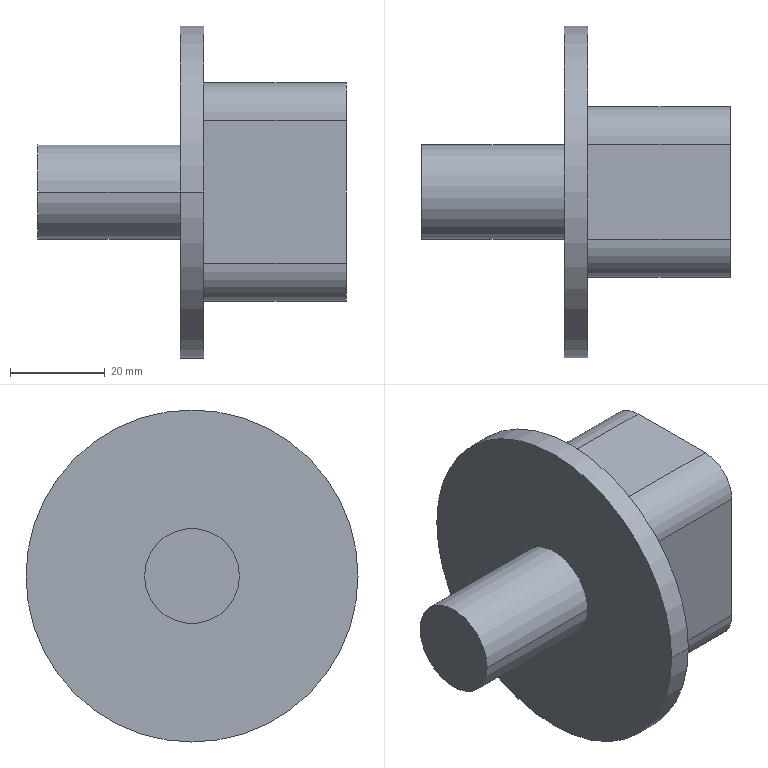Part | SolidWorks | features Extrusion 1, Revolution 1 | 1 solid | 16 faces | box 65 x 70 x 70 mm | volume 76699 mm3 | cylinder 8 | plane 8 | commonest cylinder face diameters 16 x4 20 x2 70 x2
STEP:
#1=CARTESIAN_POINT('',(-35.,-10.,0.));
#2=VERTEX_POINT('',#1);
#3=CARTESIAN_POINT('',(-35.,10.,0.));
#4=VERTEX_POINT('',#3);
#5=CARTESIAN_POINT('',(-35.,0.,0.));
#6=DIRECTION('',(-1.,0.,0.));
#7=DIRECTION('',(0.,-1.,0.));
#8=AXIS2_PLACEMENT_3D('',#5,#6,#7);
#9=CIRCLE('',#8,10.);
#10=EDGE_CURVE('',#2,#4,#9,.T.);
#11=ORIENTED_EDGE('',*,*,#10,.T.);
#12=CARTESIAN_POINT('',(-65.,10.,0.));
#13=VERTEX_POINT('',#12);
#14=CARTESIAN_POINT('',(-65.,10.,0.));
#15=DIRECTION('',(-1.,0.,0.));
#16=VECTOR('',#15,1000.);
#17=LINE('',#14,#16);
#18=EDGE_CURVE('',#4,#13,#17,.T.);
#19=ORIENTED_EDGE('',*,*,#18,.T.);
#20=CARTESIAN_POINT('',(-65.,-10.,0.));
#21=VERTEX_POINT('',#20);
#22=CARTESIAN_POINT('',(-65.,0.,0.));
#23=DIRECTION('',(-1.,0.,0.));
#24=DIRECTION('',(0.,-1.,0.));
#25=AXIS2_PLACEMENT_3D('',#22,#23,#24);
#26=CIRCLE('',#25,10.);
#27=EDGE_CURVE('',#21,#13,#26,.T.);
#28=ORIENTED_EDGE('',*,*,#27,.F.);
#29=CARTESIAN_POINT('',(-65.,-10.,0.));
#30=DIRECTION('',(-1.,0.,0.));
#31=VECTOR('',#30,1000.);
#32=LINE('',#29,#31);
#33=EDGE_CURVE('',#2,#21,#32,.T.);
#34=ORIENTED_EDGE('',*,*,#33,.F.);
#35=EDGE_LOOP('',(#11,#19,#28,#34));
#36=FACE_OUTER_BOUND('',#35,.T.);
#37=CARTESIAN_POINT('',(-65.,0.,0.));
#38=DIRECTION('',(-1.,0.,0.));
#39=DIRECTION('',(0.,-1.,0.));
#40=AXIS2_PLACEMENT_3D('',#37,#38,#39);
#41=CYLINDRICAL_SURFACE('',#40,10.);
#42=ADVANCED_FACE('',(#36),#41,.T.);
#43=CARTESIAN_POINT('',(-30.,-35.,0.));
#44=VERTEX_POINT('',#43);
#45=CARTESIAN_POINT('',(-30.,35.,0.));
#46=VERTEX_POINT('',#45);
#47=CARTESIAN_POINT('',(-30.,0.,0.));
#48=DIRECTION('',(-1.,0.,0.));
#49=DIRECTION('',(0.,-1.,0.));
#50=AXIS2_PLACEMENT_3D('',#47,#48,#49);
#51=CIRCLE('',#50,35.);
#52=EDGE_CURVE('',#44,#46,#51,.T.);
#53=ORIENTED_EDGE('',*,*,#52,.T.);
#54=CARTESIAN_POINT('',(-35.,35.,0.));
#55=VERTEX_POINT('',#54);
#56=CARTESIAN_POINT('',(-65.,35.,0.));
#57=DIRECTION('',(-1.,0.,0.));
#58=VECTOR('',#57,1000.);
#59=LINE('',#56,#58);
#60=EDGE_CURVE('',#46,#55,#59,.T.);
#61=ORIENTED_EDGE('',*,*,#60,.T.);
#62=CARTESIAN_POINT('',(-35.,-35.,0.));
#63=VERTEX_POINT('',#62);
#64=CARTESIAN_POINT('',(-35.,0.,0.));
#65=DIRECTION('',(-1.,0.,0.));
#66=DIRECTION('',(0.,-1.,0.));
#67=AXIS2_PLACEMENT_3D('',#64,#65,#66);
#68=CIRCLE('',#67,35.);
#69=EDGE_CURVE('',#63,#55,#68,.T.);
#70=ORIENTED_EDGE('',*,*,#69,.F.);
#71=CARTESIAN_POINT('',(-65.,-35.,0.));
#72=DIRECTION('',(-1.,0.,0.));
#73=VECTOR('',#72,1000.);
#74=LINE('',#71,#73);
#75=EDGE_CURVE('',#44,#63,#74,.T.);
#76=ORIENTED_EDGE('',*,*,#75,.F.);
#77=EDGE_LOOP('',(#53,#61,#70,#76));
#78=FACE_OUTER_BOUND('',#77,.T.);
#79=CARTESIAN_POINT('',(-65.,0.,0.));
#80=DIRECTION('',(-1.,0.,0.));
#81=DIRECTION('',(0.,-1.,0.));
#82=AXIS2_PLACEMENT_3D('',#79,#80,#81);
#83=CYLINDRICAL_SURFACE('',#82,35.);
#84=ADVANCED_FACE('',(#78),#83,.T.);
#85=CARTESIAN_POINT('',(0.,-10.,23.));
#86=VERTEX_POINT('',#85);
#87=CARTESIAN_POINT('',(0.,-18.,15.));
#88=VERTEX_POINT('',#87);
#89=CARTESIAN_POINT('',(0.,-10.,15.));
#90=DIRECTION('',(1.,0.,0.));
#91=DIRECTION('',(0.,0.,-1.));
#92=AXIS2_PLACEMENT_3D('',#89,#90,#91);
#93=CIRCLE('',#92,8.);
#94=EDGE_CURVE('',#86,#88,#93,.T.);
#95=ORIENTED_EDGE('',*,*,#94,.F.);
#96=CARTESIAN_POINT('',(-30.,-10.,23.));
#97=VERTEX_POINT('',#96);
#98=CARTESIAN_POINT('',(-30.,-10.,23.));
#99=DIRECTION('',(1.,0.,0.));
#100=VECTOR('',#99,1000.);
#101=LINE('',#98,#100);
#102=EDGE_CURVE('',#97,#86,#101,.T.);
#103=ORIENTED_EDGE('',*,*,#102,.F.);
#104=CARTESIAN_POINT('',(-30.,-18.,15.));
#105=VERTEX_POINT('',#104);
#106=CARTESIAN_POINT('',(-30.,-10.,15.));
#107=DIRECTION('',(1.,0.,0.));
#108=DIRECTION('',(0.,0.,-1.));
#109=AXIS2_PLACEMENT_3D('',#106,#107,#108);
#110=CIRCLE('',#109,8.);
#111=EDGE_CURVE('',#97,#105,#110,.T.);
#112=ORIENTED_EDGE('',*,*,#111,.T.);
#113=CARTESIAN_POINT('',(-30.,-18.,15.));
#114=DIRECTION('',(1.,0.,0.));
#115=VECTOR('',#114,1000.);
#116=LINE('',#113,#115);
#117=EDGE_CURVE('',#105,#88,#116,.T.);
#118=ORIENTED_EDGE('',*,*,#117,.T.);
#119=EDGE_LOOP('',(#95,#103,#112,#118));
#120=FACE_OUTER_BOUND('',#119,.T.);
#121=CARTESIAN_POINT('',(-30.,-10.,15.));
#122=DIRECTION('',(1.,0.,0.));
#123=DIRECTION('',(0.,0.,-1.));
#124=AXIS2_PLACEMENT_3D('',#121,#122,#123);
#125=CYLINDRICAL_SURFACE('',#124,8.);
#126=ADVANCED_FACE('',(#120),#125,.T.);
#127=CARTESIAN_POINT('',(0.,10.,23.));
#128=VERTEX_POINT('',#127);
#129=CARTESIAN_POINT('',(0.,10.,23.));
#130=DIRECTION('',(0.,-1.,0.));
#131=VECTOR('',#130,1000.);
#132=LINE('',#129,#131);
#133=EDGE_CURVE('',#128,#86,#132,.T.);
#134=ORIENTED_EDGE('',*,*,#133,.F.);
#135=CARTESIAN_POINT('',(-30.,10.,23.));
#136=VERTEX_POINT('',#135);
#137=CARTESIAN_POINT('',(-30.,10.,23.));
#138=DIRECTION('',(1.,0.,0.));
#139=VECTOR('',#138,1000.);
#140=LINE('',#137,#139);
#141=EDGE_CURVE('',#136,#128,#140,.T.);
#142=ORIENTED_EDGE('',*,*,#141,.F.);
#143=CARTESIAN_POINT('',(-30.,10.,23.));
#144=DIRECTION('',(0.,-1.,0.));
#145=VECTOR('',#144,1000.);
#146=LINE('',#143,#145);
#147=EDGE_CURVE('',#136,#97,#146,.T.);
#148=ORIENTED_EDGE('',*,*,#147,.T.);
#149=ORIENTED_EDGE('',*,*,#102,.T.);
#150=EDGE_LOOP('',(#134,#142,#148,#149));
#151=FACE_OUTER_BOUND('',#150,.T.);
#152=CARTESIAN_POINT('',(-30.,10.,23.));
#153=DIRECTION('',(0.,0.,1.));
#154=DIRECTION('',(1.,0.,0.));
#155=AXIS2_PLACEMENT_3D('',#152,#153,#154);
#156=PLANE('',#155);
#157=ADVANCED_FACE('',(#151),#156,.T.);
#158=CARTESIAN_POINT('',(0.,18.,15.));
#159=VERTEX_POINT('',#158);
#160=CARTESIAN_POINT('',(0.,10.,15.));
#161=DIRECTION('',(1.,0.,0.));
#162=DIRECTION('',(0.,0.,-1.));
#163=AXIS2_PLACEMENT_3D('',#160,#161,#162);
#164=CIRCLE('',#163,8.);
#165=EDGE_CURVE('',#159,#128,#164,.T.);
#166=ORIENTED_EDGE('',*,*,#165,.F.);
#167=CARTESIAN_POINT('',(-30.,18.,15.));
#168=VERTEX_POINT('',#167);
#169=CARTESIAN_POINT('',(-30.,18.,15.));
#170=DIRECTION('',(1.,0.,0.));
#171=VECTOR('',#170,1000.);
#172=LINE('',#169,#171);
#173=EDGE_CURVE('',#168,#159,#172,.T.);
#174=ORIENTED_EDGE('',*,*,#173,.F.);
#175=CARTESIAN_POINT('',(-30.,10.,15.));
#176=DIRECTION('',(1.,0.,0.));
#177=DIRECTION('',(0.,0.,-1.));
#178=AXIS2_PLACEMENT_3D('',#175,#176,#177);
#179=CIRCLE('',#178,8.);
#180=EDGE_CURVE('',#168,#136,#179,.T.);
#181=ORIENTED_EDGE('',*,*,#180,.T.);
#182=ORIENTED_EDGE('',*,*,#141,.T.);
#183=EDGE_LOOP('',(#166,#174,#181,#182));
#184=FACE_OUTER_BOUND('',#183,.T.);
#185=CARTESIAN_POINT('',(-30.,10.,15.));
#186=DIRECTION('',(1.,0.,0.));
#187=DIRECTION('',(0.,0.,-1.));
#188=AXIS2_PLACEMENT_3D('',#185,#186,#187);
#189=CYLINDRICAL_SURFACE('',#188,8.);
#190=ADVANCED_FACE('',(#184),#189,.T.);
#191=CARTESIAN_POINT('',(0.,18.,-15.));
#192=VERTEX_POINT('',#191);
#193=CARTESIAN_POINT('',(0.,18.,15.));
#194=DIRECTION('',(0.,0.,1.));
#195=VECTOR('',#194,1000.);
#196=LINE('',#193,#195);
#197=EDGE_CURVE('',#192,#159,#196,.T.);
#198=ORIENTED_EDGE('',*,*,#197,.F.);
#199=CARTESIAN_POINT('',(-30.,18.,-15.));
#200=VERTEX_POINT('',#199);
#201=CARTESIAN_POINT('',(-30.,18.,-15.));
#202=DIRECTION('',(1.,0.,0.));
#203=VECTOR('',#202,1000.);
#204=LINE('',#201,#203);
#205=EDGE_CURVE('',#200,#192,#204,.T.);
#206=ORIENTED_EDGE('',*,*,#205,.F.);
#207=CARTESIAN_POINT('',(-30.,18.,15.));
#208=DIRECTION('',(0.,0.,1.));
#209=VECTOR('',#208,1000.);
#210=LINE('',#207,#209);
#211=EDGE_CURVE('',#200,#168,#210,.T.);
#212=ORIENTED_EDGE('',*,*,#211,.T.);
#213=ORIENTED_EDGE('',*,*,#173,.T.);
#214=EDGE_LOOP('',(#198,#206,#212,#213));
#215=FACE_OUTER_BOUND('',#214,.T.);
#216=CARTESIAN_POINT('',(-30.,18.,15.));
#217=DIRECTION('',(0.,1.,0.));
#218=DIRECTION('',(0.,0.,1.));
#219=AXIS2_PLACEMENT_3D('',#216,#217,#218);
#220=PLANE('',#219);
#221=ADVANCED_FACE('',(#215),#220,.T.);
#222=CARTESIAN_POINT('',(0.,10.,-23.));
#223=VERTEX_POINT('',#222);
#224=CARTESIAN_POINT('',(0.,10.,-15.));
#225=DIRECTION('',(1.,0.,0.));
#226=DIRECTION('',(0.,0.,1.));
#227=AXIS2_PLACEMENT_3D('',#224,#225,#226);
#228=CIRCLE('',#227,8.);
#229=EDGE_CURVE('',#223,#192,#228,.T.);
#230=ORIENTED_EDGE('',*,*,#229,.F.);
#231=CARTESIAN_POINT('',(-30.,10.,-23.));
#232=VERTEX_POINT('',#231);
#233=CARTESIAN_POINT('',(-30.,10.,-23.));
#234=DIRECTION('',(1.,0.,0.));
#235=VECTOR('',#234,1000.);
#236=LINE('',#233,#235);
#237=EDGE_CURVE('',#232,#223,#236,.T.);
#238=ORIENTED_EDGE('',*,*,#237,.F.);
#239=CARTESIAN_POINT('',(-30.,10.,-15.));
#240=DIRECTION('',(1.,0.,0.));
#241=DIRECTION('',(0.,0.,1.));
#242=AXIS2_PLACEMENT_3D('',#239,#240,#241);
#243=CIRCLE('',#242,8.);
#244=EDGE_CURVE('',#232,#200,#243,.T.);
#245=ORIENTED_EDGE('',*,*,#244,.T.);
#246=ORIENTED_EDGE('',*,*,#205,.T.);
#247=EDGE_LOOP('',(#230,#238,#245,#246));
#248=FACE_OUTER_BOUND('',#247,.T.);
#249=CARTESIAN_POINT('',(-30.,10.,-15.));
#250=DIRECTION('',(1.,0.,0.));
#251=DIRECTION('',(0.,0.,-1.));
#252=AXIS2_PLACEMENT_3D('',#249,#250,#251);
#253=CYLINDRICAL_SURFACE('',#252,8.);
#254=ADVANCED_FACE('',(#248),#253,.T.);
#255=CARTESIAN_POINT('',(0.,-10.,-23.));
#256=VERTEX_POINT('',#255);
#257=CARTESIAN_POINT('',(0.,10.,-23.));
#258=DIRECTION('',(0.,1.,0.));
#259=VECTOR('',#258,1000.);
#260=LINE('',#257,#259);
#261=EDGE_CURVE('',#256,#223,#260,.T.);
#262=ORIENTED_EDGE('',*,*,#261,.F.);
#263=CARTESIAN_POINT('',(-30.,-10.,-23.));
#264=VERTEX_POINT('',#263);
#265=CARTESIAN_POINT('',(-30.,-10.,-23.));
#266=DIRECTION('',(1.,0.,0.));
#267=VECTOR('',#266,1000.);
#268=LINE('',#265,#267);
#269=EDGE_CURVE('',#264,#256,#268,.T.);
#270=ORIENTED_EDGE('',*,*,#269,.F.);
#271=CARTESIAN_POINT('',(-30.,10.,-23.));
#272=DIRECTION('',(0.,1.,0.));
#273=VECTOR('',#272,1000.);
#274=LINE('',#271,#273);
#275=EDGE_CURVE('',#264,#232,#274,.T.);
#276=ORIENTED_EDGE('',*,*,#275,.T.);
#277=ORIENTED_EDGE('',*,*,#237,.T.);
#278=EDGE_LOOP('',(#262,#270,#276,#277));
#279=FACE_OUTER_BOUND('',#278,.T.);
#280=CARTESIAN_POINT('',(-30.,10.,-23.));
#281=DIRECTION('',(0.,0.,-1.));
#282=DIRECTION('',(-1.,0.,0.));
#283=AXIS2_PLACEMENT_3D('',#280,#281,#282);
#284=PLANE('',#283);
#285=ADVANCED_FACE('',(#279),#284,.T.);
#286=CARTESIAN_POINT('',(0.,-18.,-15.));
#287=VERTEX_POINT('',#286);
#288=CARTESIAN_POINT('',(0.,-10.,-15.));
#289=DIRECTION('',(1.,0.,0.));
#290=DIRECTION('',(0.,0.,-1.));
#291=AXIS2_PLACEMENT_3D('',#288,#289,#290);
#292=CIRCLE('',#291,8.);
#293=EDGE_CURVE('',#287,#256,#292,.T.);
#294=ORIENTED_EDGE('',*,*,#293,.F.);
#295=CARTESIAN_POINT('',(-30.,-18.,-15.));
#296=VERTEX_POINT('',#295);
#297=CARTESIAN_POINT('',(-30.,-18.,-15.));
#298=DIRECTION('',(1.,0.,0.));
#299=VECTOR('',#298,1000.);
#300=LINE('',#297,#299);
#301=EDGE_CURVE('',#296,#287,#300,.T.);
#302=ORIENTED_EDGE('',*,*,#301,.F.);
#303=CARTESIAN_POINT('',(-30.,-10.,-15.));
#304=DIRECTION('',(1.,0.,0.));
#305=DIRECTION('',(0.,0.,-1.));
#306=AXIS2_PLACEMENT_3D('',#303,#304,#305);
#307=CIRCLE('',#306,8.);
#308=EDGE_CURVE('',#296,#264,#307,.T.);
#309=ORIENTED_EDGE('',*,*,#308,.T.);
#310=ORIENTED_EDGE('',*,*,#269,.T.);
#311=EDGE_LOOP('',(#294,#302,#309,#310));
#312=FACE_OUTER_BOUND('',#311,.T.);
#313=CARTESIAN_POINT('',(-30.,-10.,-15.));
#314=DIRECTION('',(1.,0.,0.));
#315=DIRECTION('',(0.,0.,-1.));
#316=AXIS2_PLACEMENT_3D('',#313,#314,#315);
#317=CYLINDRICAL_SURFACE('',#316,8.);
#318=ADVANCED_FACE('',(#312),#317,.T.);
#319=CARTESIAN_POINT('',(0.,-18.,15.));
#320=DIRECTION('',(0.,0.,-1.));
#321=VECTOR('',#320,1000.);
#322=LINE('',#319,#321);
#323=EDGE_CURVE('',#88,#287,#322,.T.);
#324=ORIENTED_EDGE('',*,*,#323,.F.);
#325=ORIENTED_EDGE('',*,*,#117,.F.);
#326=CARTESIAN_POINT('',(-30.,-18.,15.));
#327=DIRECTION('',(0.,0.,-1.));
#328=VECTOR('',#327,1000.);
#329=LINE('',#326,#328);
#330=EDGE_CURVE('',#105,#296,#329,.T.);
#331=ORIENTED_EDGE('',*,*,#330,.T.);
#332=ORIENTED_EDGE('',*,*,#301,.T.);
#333=EDGE_LOOP('',(#324,#325,#331,#332));
#334=FACE_OUTER_BOUND('',#333,.T.);
#335=CARTESIAN_POINT('',(-30.,-18.,15.));
#336=DIRECTION('',(0.,-1.,0.));
#337=DIRECTION('',(0.,0.,-1.));
#338=AXIS2_PLACEMENT_3D('',#335,#336,#337);
#339=PLANE('',#338);
#340=ADVANCED_FACE('',(#334),#339,.T.);
#341=ORIENTED_EDGE('',*,*,#94,.T.);
#342=ORIENTED_EDGE('',*,*,#323,.T.);
#343=ORIENTED_EDGE('',*,*,#293,.T.);
#344=ORIENTED_EDGE('',*,*,#261,.T.);
#345=ORIENTED_EDGE('',*,*,#229,.T.);
#346=ORIENTED_EDGE('',*,*,#197,.T.);
#347=ORIENTED_EDGE('',*,*,#165,.T.);
#348=ORIENTED_EDGE('',*,*,#133,.T.);
#349=EDGE_LOOP('',(#341,#342,#343,#344,#345,#346,#347,#348));
#350=FACE_OUTER_BOUND('',#349,.T.);
#351=CARTESIAN_POINT('',(0.,-10.,15.));
#352=DIRECTION('',(1.,0.,0.));
#353=DIRECTION('',(0.,0.,-1.));
#354=AXIS2_PLACEMENT_3D('',#351,#352,#353);
#355=PLANE('',#354);
#356=ADVANCED_FACE('',(#350),#355,.T.);
#357=ORIENTED_EDGE('',*,*,#111,.F.);
#358=ORIENTED_EDGE('',*,*,#147,.F.);
#359=ORIENTED_EDGE('',*,*,#180,.F.);
#360=ORIENTED_EDGE('',*,*,#211,.F.);
#361=ORIENTED_EDGE('',*,*,#244,.F.);
#362=ORIENTED_EDGE('',*,*,#275,.F.);
#363=ORIENTED_EDGE('',*,*,#308,.F.);
#364=ORIENTED_EDGE('',*,*,#330,.F.);
#365=EDGE_LOOP('',(#357,#358,#359,#360,#361,#362,#363,#364));
#366=FACE_BOUND('',#365,.T.);
#367=ORIENTED_EDGE('',*,*,#52,.F.);
#368=CARTESIAN_POINT('',(-30.,0.,0.));
#369=DIRECTION('',(-1.,0.,0.));
#370=DIRECTION('',(0.,-1.,0.));
#371=AXIS2_PLACEMENT_3D('',#368,#369,#370);
#372=CIRCLE('',#371,35.);
#373=EDGE_CURVE('',#46,#44,#372,.T.);
#374=ORIENTED_EDGE('',*,*,#373,.F.);
#375=EDGE_LOOP('',(#367,#374));
#376=FACE_OUTER_BOUND('',#375,.T.);
#377=CARTESIAN_POINT('',(-30.,0.,0.));
#378=DIRECTION('',(-1.,0.,0.));
#379=DIRECTION('',(0.,-1.,0.));
#380=AXIS2_PLACEMENT_3D('',#377,#378,#379);
#381=PLANE('',#380);
#382=ADVANCED_FACE('',(#366,#376),#381,.F.);
#383=ORIENTED_EDGE('',*,*,#60,.F.);
#384=ORIENTED_EDGE('',*,*,#373,.T.);
#385=ORIENTED_EDGE('',*,*,#75,.T.);
#386=CARTESIAN_POINT('',(-35.,0.,0.));
#387=DIRECTION('',(-1.,0.,0.));
#388=DIRECTION('',(0.,-1.,0.));
#389=AXIS2_PLACEMENT_3D('',#386,#387,#388);
#390=CIRCLE('',#389,35.);
#391=EDGE_CURVE('',#55,#63,#390,.T.);
#392=ORIENTED_EDGE('',*,*,#391,.F.);
#393=EDGE_LOOP('',(#383,#384,#385,#392));
#394=FACE_OUTER_BOUND('',#393,.T.);
#395=CARTESIAN_POINT('',(-65.,0.,0.));
#396=DIRECTION('',(-1.,0.,0.));
#397=DIRECTION('',(0.,-1.,0.));
#398=AXIS2_PLACEMENT_3D('',#395,#396,#397);
#399=CYLINDRICAL_SURFACE('',#398,35.);
#400=ADVANCED_FACE('',(#394),#399,.T.);
#401=ORIENTED_EDGE('',*,*,#10,.F.);
#402=CARTESIAN_POINT('',(-35.,0.,0.));
#403=DIRECTION('',(-1.,0.,0.));
#404=DIRECTION('',(0.,-1.,0.));
#405=AXIS2_PLACEMENT_3D('',#402,#403,#404);
#406=CIRCLE('',#405,10.);
#407=EDGE_CURVE('',#4,#2,#406,.T.);
#408=ORIENTED_EDGE('',*,*,#407,.F.);
#409=EDGE_LOOP('',(#401,#408));
#410=FACE_BOUND('',#409,.T.);
#411=ORIENTED_EDGE('',*,*,#69,.T.);
#412=ORIENTED_EDGE('',*,*,#391,.T.);
#413=EDGE_LOOP('',(#411,#412));
#414=FACE_OUTER_BOUND('',#413,.T.);
#415=CARTESIAN_POINT('',(-35.,35.,0.));
#416=DIRECTION('',(1.,0.,0.));
#417=DIRECTION('',(0.,1.,0.));
#418=AXIS2_PLACEMENT_3D('',#415,#416,#417);
#419=PLANE('',#418);
#420=ADVANCED_FACE('',(#410,#414),#419,.F.);
#421=ORIENTED_EDGE('',*,*,#18,.F.);
#422=ORIENTED_EDGE('',*,*,#407,.T.);
#423=ORIENTED_EDGE('',*,*,#33,.T.);
#424=CARTESIAN_POINT('',(-65.,0.,0.));
#425=DIRECTION('',(-1.,0.,0.));
#426=DIRECTION('',(0.,-1.,0.));
#427=AXIS2_PLACEMENT_3D('',#424,#425,#426);
#428=CIRCLE('',#427,10.);
#429=EDGE_CURVE('',#13,#21,#428,.T.);
#430=ORIENTED_EDGE('',*,*,#429,.F.);
#431=EDGE_LOOP('',(#421,#422,#423,#430));
#432=FACE_OUTER_BOUND('',#431,.T.);
#433=CARTESIAN_POINT('',(-65.,0.,0.));
#434=DIRECTION('',(-1.,0.,0.));
#435=DIRECTION('',(0.,-1.,0.));
#436=AXIS2_PLACEMENT_3D('',#433,#434,#435);
#437=CYLINDRICAL_SURFACE('',#436,10.);
#438=ADVANCED_FACE('',(#432),#437,.T.);
#439=ORIENTED_EDGE('',*,*,#27,.T.);
#440=ORIENTED_EDGE('',*,*,#429,.T.);
#441=EDGE_LOOP('',(#439,#440));
#442=FACE_OUTER_BOUND('',#441,.T.);
#443=CARTESIAN_POINT('',(-65.,10.,0.));
#444=DIRECTION('',(1.,0.,0.));
#445=DIRECTION('',(0.,1.,0.));
#446=AXIS2_PLACEMENT_3D('',#443,#444,#445);
#447=PLANE('',#446);
#448=ADVANCED_FACE('',(#442),#447,.F.);
#449=CLOSED_SHELL('',(#42,#84,#126,#157,#190,#221,#254,#285,#318,#340,#356,#382,#400,#420,#438,#448));
#450=MANIFOLD_SOLID_BREP('',#449);
#451=CARTESIAN_POINT('',(0.,0.,0.));
#452=DIRECTION('',(0.,0.,1.));
#453=DIRECTION('',(1.,0.,0.));
#454=AXIS2_PLACEMENT_3D('',#451,#452,#453);
#455=(LENGTH_UNIT()NAMED_UNIT(*)SI_UNIT(.MILLI.,.METRE.));
#456=UNCERTAINTY_MEASURE_WITH_UNIT(LENGTH_MEASURE(0.00001),#455,'','');
#457=(NAMED_UNIT(*)PLANE_ANGLE_UNIT()SI_UNIT($,.RADIAN.));
#458=(NAMED_UNIT(*)SI_UNIT($,.STERADIAN.)SOLID_ANGLE_UNIT());
#459=(GEOMETRIC_REPRESENTATION_CONTEXT(3)GLOBAL_UNCERTAINTY_ASSIGNED_CONTEXT((#456))GLOBAL_UNIT_ASSIGNED_CONTEXT((#455,#457,#458))REPRESENTATION_CONTEXT('',''));
#460=ADVANCED_BREP_SHAPE_REPRESENTATION('',(#450,#454),#459);